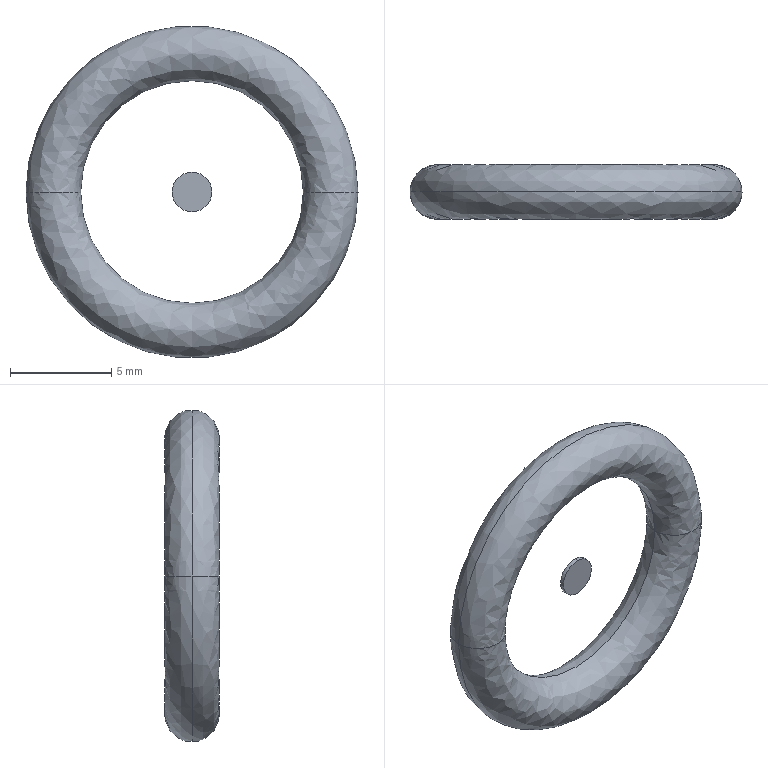Part | STEP file | 20501 | 2 solids | 8 faces | box 16.4 x 2.7 x 16.4 mm | volume 247.033 mm3 | spline 4 | cylinder 2 | plane 2 | commonest cylinder face diameters 1.965 x2
STEP:
#1=CARTESIAN_POINT('',(0.,0.,0.));
#2=DIRECTION('',(0.,0.,1.));
#3=DIRECTION('',(1.,0.,0.));
#4=AXIS2_PLACEMENT_3D('',#1,#2,#3);
#5=CARTESIAN_POINT('',(-5.5,0.,0.));
#6=VERTEX_POINT('',#5);
#7=CARTESIAN_POINT('',(5.5,0.,0.));
#8=VERTEX_POINT('',#7);
#9=CARTESIAN_POINT('',(0.,0.,0.));
#10=DIRECTION('',(0.,1.,0.));
#11=DIRECTION('',(1.,0.,0.));
#12=AXIS2_PLACEMENT_3D('',#9,#10,#11);
#13=CIRCLE('',#12,5.5);
#14=CARTESIAN_POINT('',(-5.5,0.,0.));
#15=CARTESIAN_POINT('',(-5.5,0.,11.));
#16=CARTESIAN_POINT('',(5.5,0.,11.));
#17=CARTESIAN_POINT('',(5.5,0.,0.));
#18=CARTESIAN_POINT('',(-5.5,2.7,0.));
#19=CARTESIAN_POINT('',(-5.5,2.7,11.));
#20=CARTESIAN_POINT('',(5.5,2.7,11.));
#21=CARTESIAN_POINT('',(5.5,2.7,0.));
#22=CARTESIAN_POINT('',(-8.2,2.7,0.));
#23=CARTESIAN_POINT('',(-8.2,2.7,16.4));
#24=CARTESIAN_POINT('',(8.2,2.7,16.4));
#25=CARTESIAN_POINT('',(8.2,2.7,0.));
#26=CARTESIAN_POINT('',(-8.2,0.,0.));
#27=CARTESIAN_POINT('',(-8.2,0.,16.4));
#28=CARTESIAN_POINT('',(8.2,0.,16.4));
#29=CARTESIAN_POINT('',(8.2,0.,0.));
#30=(BOUNDED_SURFACE()B_SPLINE_SURFACE(3,3,((#14,#15,#16,#17),(#18,#19,#20,#21),(#22,#23,#24,#25),(#26,#27,#28,#29)),.UNSPECIFIED.,.F.,.F.,.F.)B_SPLINE_SURFACE_WITH_KNOTS((4,4),(4,4),(0.,1.),(0.,1.),.PIECEWISE_BEZIER_KNOTS.)GEOMETRIC_REPRESENTATION_ITEM()RATIONAL_B_SPLINE_SURFACE(((1.,0.3333,0.3333,1.),(0.3333,0.1111,0.1111,0.3333),(0.3333,0.1111,0.1111,0.3333),(1.,0.3333,0.3333,1.)))REPRESENTATION_ITEM('')SURFACE());
#31=CARTESIAN_POINT('',(0.,0.));
#32=CARTESIAN_POINT('',(0.,0.02375));
#33=CARTESIAN_POINT('',(0.,0.06805));
#34=CARTESIAN_POINT('',(0.,0.1267));
#35=CARTESIAN_POINT('',(0.,0.1794));
#36=CARTESIAN_POINT('',(0.,0.2276));
#37=CARTESIAN_POINT('',(0.,0.2721));
#38=CARTESIAN_POINT('',(0.,0.3139));
#39=CARTESIAN_POINT('',(0.,0.3535));
#40=CARTESIAN_POINT('',(0.,0.3914));
#41=CARTESIAN_POINT('',(0.,0.4282));
#42=CARTESIAN_POINT('',(0.,0.4643));
#43=CARTESIAN_POINT('',(0.,0.5));
#44=CARTESIAN_POINT('',(0.,0.5357));
#45=CARTESIAN_POINT('',(0.,0.5718));
#46=CARTESIAN_POINT('',(0.,0.6086));
#47=CARTESIAN_POINT('',(0.,0.6465));
#48=CARTESIAN_POINT('',(0.,0.6861));
#49=CARTESIAN_POINT('',(0.,0.7279));
#50=CARTESIAN_POINT('',(0.,0.7724));
#51=CARTESIAN_POINT('',(0.,0.8206));
#52=CARTESIAN_POINT('',(0.,0.8733));
#53=CARTESIAN_POINT('',(0.,0.9319));
#54=CARTESIAN_POINT('',(0.,0.9763));
#55=CARTESIAN_POINT('',(0.,1.));
#56=B_SPLINE_CURVE_WITH_KNOTS('',3,(#31,#32,#33,#34,#35,#36,#37,#38,#39,#40,#41,#42,#43,#44,#45,#46,#47,#48,#49,#50,#51,#52,#53,#54,#55),.UNSPECIFIED.,.F.,.F.,(4,1,1,1,1,1,1,1,1,1,1,1,1,1,1,1,1,1,1,1,1,1,4),(3.142,3.284,3.427,3.57,3.713,3.856,3.998,4.141,4.284,4.427,4.57,4.712,4.855,4.998,5.141,5.284,5.426,5.569,5.712,5.855,5.998,6.14,6.283),.QUASI_UNIFORM_KNOTS.);
#57=(GEOMETRIC_REPRESENTATION_CONTEXT(2)PARAMETRIC_REPRESENTATION_CONTEXT()REPRESENTATION_CONTEXT('',''));
#58=DEFINITIONAL_REPRESENTATION('',(#56),#57);
#59=PCURVE('',#30,#58);
#60=CARTESIAN_POINT('',(-8.2,0.,0.));
#61=CARTESIAN_POINT('',(-8.2,0.,16.4));
#62=CARTESIAN_POINT('',(8.2,0.,16.4));
#63=CARTESIAN_POINT('',(8.2,0.,0.));
#64=CARTESIAN_POINT('',(-8.2,-2.7,0.));
#65=CARTESIAN_POINT('',(-8.2,-2.7,16.4));
#66=CARTESIAN_POINT('',(8.2,-2.7,16.4));
#67=CARTESIAN_POINT('',(8.2,-2.7,0.));
#68=CARTESIAN_POINT('',(-5.5,-2.7,0.));
#69=CARTESIAN_POINT('',(-5.5,-2.7,11.));
#70=CARTESIAN_POINT('',(5.5,-2.7,11.));
#71=CARTESIAN_POINT('',(5.5,-2.7,0.));
#72=CARTESIAN_POINT('',(-5.5,0.,0.));
#73=CARTESIAN_POINT('',(-5.5,0.,11.));
#74=CARTESIAN_POINT('',(5.5,0.,11.));
#75=CARTESIAN_POINT('',(5.5,0.,0.));
#76=(BOUNDED_SURFACE()B_SPLINE_SURFACE(3,3,((#60,#61,#62,#63),(#64,#65,#66,#67),(#68,#69,#70,#71),(#72,#73,#74,#75)),.UNSPECIFIED.,.F.,.F.,.F.)B_SPLINE_SURFACE_WITH_KNOTS((4,4),(4,4),(0.,1.),(0.,1.),.PIECEWISE_BEZIER_KNOTS.)GEOMETRIC_REPRESENTATION_ITEM()RATIONAL_B_SPLINE_SURFACE(((1.,0.3333,0.3333,1.),(0.3333,0.1111,0.1111,0.3333),(0.3333,0.1111,0.1111,0.3333),(1.,0.3333,0.3333,1.)))REPRESENTATION_ITEM('')SURFACE());
#77=CARTESIAN_POINT('',(1.,0.));
#78=CARTESIAN_POINT('',(1.,0.02375));
#79=CARTESIAN_POINT('',(1.,0.06805));
#80=CARTESIAN_POINT('',(1.,0.1267));
#81=CARTESIAN_POINT('',(1.,0.1794));
#82=CARTESIAN_POINT('',(1.,0.2276));
#83=CARTESIAN_POINT('',(1.,0.2721));
#84=CARTESIAN_POINT('',(1.,0.3139));
#85=CARTESIAN_POINT('',(1.,0.3535));
#86=CARTESIAN_POINT('',(1.,0.3914));
#87=CARTESIAN_POINT('',(1.,0.4282));
#88=CARTESIAN_POINT('',(1.,0.4643));
#89=CARTESIAN_POINT('',(1.,0.5));
#90=CARTESIAN_POINT('',(1.,0.5357));
#91=CARTESIAN_POINT('',(1.,0.5718));
#92=CARTESIAN_POINT('',(1.,0.6086));
#93=CARTESIAN_POINT('',(1.,0.6465));
#94=CARTESIAN_POINT('',(1.,0.6861));
#95=CARTESIAN_POINT('',(1.,0.7279));
#96=CARTESIAN_POINT('',(1.,0.7724));
#97=CARTESIAN_POINT('',(1.,0.8206));
#98=CARTESIAN_POINT('',(1.,0.8733));
#99=CARTESIAN_POINT('',(1.,0.9319));
#100=CARTESIAN_POINT('',(1.,0.9763));
#101=CARTESIAN_POINT('',(1.,1.));
#102=B_SPLINE_CURVE_WITH_KNOTS('',3,(#77,#78,#79,#80,#81,#82,#83,#84,#85,#86,#87,#88,#89,#90,#91,#92,#93,#94,#95,#96,#97,#98,#99,#100,#101),.UNSPECIFIED.,.F.,.F.,(4,1,1,1,1,1,1,1,1,1,1,1,1,1,1,1,1,1,1,1,1,1,4),(3.142,3.284,3.427,3.57,3.713,3.856,3.998,4.141,4.284,4.427,4.57,4.712,4.855,4.998,5.141,5.284,5.426,5.569,5.712,5.855,5.998,6.14,6.283),.QUASI_UNIFORM_KNOTS.);
#103=(GEOMETRIC_REPRESENTATION_CONTEXT(2)PARAMETRIC_REPRESENTATION_CONTEXT()REPRESENTATION_CONTEXT('',''));
#104=DEFINITIONAL_REPRESENTATION('',(#102),#103);
#105=PCURVE('',#76,#104);
#106=SURFACE_CURVE('',#13,(#59,#105),.PCURVE_S1.);
#107=EDGE_CURVE('',#6,#8,#106,.T.);
#108=ORIENTED_EDGE('',*,*,#107,.F.);
#109=CARTESIAN_POINT('',(-8.2,0.,0.));
#110=VERTEX_POINT('',#109);
#111=CARTESIAN_POINT('',(-6.85,0.,0.));
#112=DIRECTION('',(0.,0.,1.));
#113=DIRECTION('',(-1.,0.,0.));
#114=AXIS2_PLACEMENT_3D('',#111,#112,#113);
#115=CIRCLE('',#114,1.35);
#116=CARTESIAN_POINT('',(0.,0.));
#117=CARTESIAN_POINT('',(0.02375,0.));
#118=CARTESIAN_POINT('',(0.06805,0.));
#119=CARTESIAN_POINT('',(0.1267,0.));
#120=CARTESIAN_POINT('',(0.1794,0.));
#121=CARTESIAN_POINT('',(0.2276,0.));
#122=CARTESIAN_POINT('',(0.2721,0.));
#123=CARTESIAN_POINT('',(0.3139,0.));
#124=CARTESIAN_POINT('',(0.3535,0.));
#125=CARTESIAN_POINT('',(0.3914,0.));
#126=CARTESIAN_POINT('',(0.4282,0.));
#127=CARTESIAN_POINT('',(0.4643,0.));
#128=CARTESIAN_POINT('',(0.5,0.));
#129=CARTESIAN_POINT('',(0.5357,0.));
#130=CARTESIAN_POINT('',(0.5718,0.));
#131=CARTESIAN_POINT('',(0.6086,0.));
#132=CARTESIAN_POINT('',(0.6465,0.));
#133=CARTESIAN_POINT('',(0.6861,0.));
#134=CARTESIAN_POINT('',(0.7279,0.));
#135=CARTESIAN_POINT('',(0.7724,0.));
#136=CARTESIAN_POINT('',(0.8206,0.));
#137=CARTESIAN_POINT('',(0.8733,0.));
#138=CARTESIAN_POINT('',(0.9319,0.));
#139=CARTESIAN_POINT('',(0.9763,0.));
#140=CARTESIAN_POINT('',(1.,0.));
#141=B_SPLINE_CURVE_WITH_KNOTS('',3,(#116,#117,#118,#119,#120,#121,#122,#123,#124,#125,#126,#127,#128,#129,#130,#131,#132,#133,#134,#135,#136,#137,#138,#139,#140),.UNSPECIFIED.,.F.,.F.,(4,1,1,1,1,1,1,1,1,1,1,1,1,1,1,1,1,1,1,1,1,1,4),(3.142,3.284,3.427,3.57,3.713,3.856,3.998,4.141,4.284,4.427,4.57,4.712,4.855,4.998,5.141,5.284,5.426,5.569,5.712,5.855,5.998,6.14,6.283),.QUASI_UNIFORM_KNOTS.);
#142=(GEOMETRIC_REPRESENTATION_CONTEXT(2)PARAMETRIC_REPRESENTATION_CONTEXT()REPRESENTATION_CONTEXT('',''));
#143=DEFINITIONAL_REPRESENTATION('',(#141),#142);
#144=PCURVE('',#30,#143);
#145=CARTESIAN_POINT('',(5.5,0.,0.));
#146=CARTESIAN_POINT('',(5.5,0.,-11.));
#147=CARTESIAN_POINT('',(-5.5,0.,-11.));
#148=CARTESIAN_POINT('',(-5.5,0.,0.));
#149=CARTESIAN_POINT('',(5.5,2.7,0.));
#150=CARTESIAN_POINT('',(5.5,2.7,-11.));
#151=CARTESIAN_POINT('',(-5.5,2.7,-11.));
#152=CARTESIAN_POINT('',(-5.5,2.7,0.));
#153=CARTESIAN_POINT('',(8.2,2.7,0.));
#154=CARTESIAN_POINT('',(8.2,2.7,-16.4));
#155=CARTESIAN_POINT('',(-8.2,2.7,-16.4));
#156=CARTESIAN_POINT('',(-8.2,2.7,0.));
#157=CARTESIAN_POINT('',(8.2,0.,0.));
#158=CARTESIAN_POINT('',(8.2,0.,-16.4));
#159=CARTESIAN_POINT('',(-8.2,0.,-16.4));
#160=CARTESIAN_POINT('',(-8.2,0.,0.));
#161=(BOUNDED_SURFACE()B_SPLINE_SURFACE(3,3,((#145,#146,#147,#148),(#149,#150,#151,#152),(#153,#154,#155,#156),(#157,#158,#159,#160)),.UNSPECIFIED.,.F.,.F.,.F.)B_SPLINE_SURFACE_WITH_KNOTS((4,4),(4,4),(0.,1.),(0.,1.),.PIECEWISE_BEZIER_KNOTS.)GEOMETRIC_REPRESENTATION_ITEM()RATIONAL_B_SPLINE_SURFACE(((1.,0.3333,0.3333,1.),(0.3333,0.1111,0.1111,0.3333),(0.3333,0.1111,0.1111,0.3333),(1.,0.3333,0.3333,1.)))REPRESENTATION_ITEM('')SURFACE());
#162=CARTESIAN_POINT('',(0.,1.));
#163=CARTESIAN_POINT('',(0.02375,1.));
#164=CARTESIAN_POINT('',(0.06805,1.));
#165=CARTESIAN_POINT('',(0.1267,1.));
#166=CARTESIAN_POINT('',(0.1794,1.));
#167=CARTESIAN_POINT('',(0.2276,1.));
#168=CARTESIAN_POINT('',(0.2721,1.));
#169=CARTESIAN_POINT('',(0.3139,1.));
#170=CARTESIAN_POINT('',(0.3535,1.));
#171=CARTESIAN_POINT('',(0.3914,1.));
#172=CARTESIAN_POINT('',(0.4282,1.));
#173=CARTESIAN_POINT('',(0.4643,1.));
#174=CARTESIAN_POINT('',(0.5,1.));
#175=CARTESIAN_POINT('',(0.5357,1.));
#176=CARTESIAN_POINT('',(0.5718,1.));
#177=CARTESIAN_POINT('',(0.6086,1.));
#178=CARTESIAN_POINT('',(0.6465,1.));
#179=CARTESIAN_POINT('',(0.6861,1.));
#180=CARTESIAN_POINT('',(0.7279,1.));
#181=CARTESIAN_POINT('',(0.7724,1.));
#182=CARTESIAN_POINT('',(0.8206,1.));
#183=CARTESIAN_POINT('',(0.8733,1.));
#184=CARTESIAN_POINT('',(0.9319,1.));
#185=CARTESIAN_POINT('',(0.9763,1.));
#186=CARTESIAN_POINT('',(1.,1.));
#187=B_SPLINE_CURVE_WITH_KNOTS('',3,(#162,#163,#164,#165,#166,#167,#168,#169,#170,#171,#172,#173,#174,#175,#176,#177,#178,#179,#180,#181,#182,#183,#184,#185,#186),.UNSPECIFIED.,.F.,.F.,(4,1,1,1,1,1,1,1,1,1,1,1,1,1,1,1,1,1,1,1,1,1,4),(3.142,3.284,3.427,3.57,3.713,3.856,3.998,4.141,4.284,4.427,4.57,4.712,4.855,4.998,5.141,5.284,5.426,5.569,5.712,5.855,5.998,6.14,6.283),.QUASI_UNIFORM_KNOTS.);
#188=(GEOMETRIC_REPRESENTATION_CONTEXT(2)PARAMETRIC_REPRESENTATION_CONTEXT()REPRESENTATION_CONTEXT('',''));
#189=DEFINITIONAL_REPRESENTATION('',(#187),#188);
#190=PCURVE('',#161,#189);
#191=SURFACE_CURVE('',#115,(#144,#190),.PCURVE_S1.);
#192=EDGE_CURVE('',#6,#110,#191,.T.);
#193=ORIENTED_EDGE('',*,*,#192,.T.);
#194=CARTESIAN_POINT('',(8.2,0.,0.));
#195=VERTEX_POINT('',#194);
#196=CARTESIAN_POINT('',(0.,0.,0.));
#197=DIRECTION('',(0.,1.,0.));
#198=DIRECTION('',(1.,0.,0.));
#199=AXIS2_PLACEMENT_3D('',#196,#197,#198);
#200=CIRCLE('',#199,8.2);
#201=CARTESIAN_POINT('',(1.,0.));
#202=CARTESIAN_POINT('',(1.,0.02375));
#203=CARTESIAN_POINT('',(1.,0.06805));
#204=CARTESIAN_POINT('',(1.,0.1267));
#205=CARTESIAN_POINT('',(1.,0.1794));
#206=CARTESIAN_POINT('',(1.,0.2276));
#207=CARTESIAN_POINT('',(1.,0.2721));
#208=CARTESIAN_POINT('',(1.,0.3139));
#209=CARTESIAN_POINT('',(1.,0.3535));
#210=CARTESIAN_POINT('',(1.,0.3914));
#211=CARTESIAN_POINT('',(1.,0.4282));
#212=CARTESIAN_POINT('',(1.,0.4643));
#213=CARTESIAN_POINT('',(1.,0.5));
#214=CARTESIAN_POINT('',(1.,0.5357));
#215=CARTESIAN_POINT('',(1.,0.5718));
#216=CARTESIAN_POINT('',(1.,0.6086));
#217=CARTESIAN_POINT('',(1.,0.6465));
#218=CARTESIAN_POINT('',(1.,0.6861));
#219=CARTESIAN_POINT('',(1.,0.7279));
#220=CARTESIAN_POINT('',(1.,0.7724));
#221=CARTESIAN_POINT('',(1.,0.8206));
#222=CARTESIAN_POINT('',(1.,0.8733));
#223=CARTESIAN_POINT('',(1.,0.9319));
#224=CARTESIAN_POINT('',(1.,0.9763));
#225=CARTESIAN_POINT('',(1.,1.));
#226=B_SPLINE_CURVE_WITH_KNOTS('',3,(#201,#202,#203,#204,#205,#206,#207,#208,#209,#210,#211,#212,#213,#214,#215,#216,#217,#218,#219,#220,#221,#222,#223,#224,#225),.UNSPECIFIED.,.F.,.F.,(4,1,1,1,1,1,1,1,1,1,1,1,1,1,1,1,1,1,1,1,1,1,4),(3.142,3.284,3.427,3.57,3.713,3.856,3.998,4.141,4.284,4.427,4.57,4.712,4.855,4.998,5.141,5.284,5.426,5.569,5.712,5.855,5.998,6.14,6.283),.QUASI_UNIFORM_KNOTS.);
#227=(GEOMETRIC_REPRESENTATION_CONTEXT(2)PARAMETRIC_REPRESENTATION_CONTEXT()REPRESENTATION_CONTEXT('',''));
#228=DEFINITIONAL_REPRESENTATION('',(#226),#227);
#229=PCURVE('',#30,#228);
#230=CARTESIAN_POINT('',(0.,0.));
#231=CARTESIAN_POINT('',(0.,0.02375));
#232=CARTESIAN_POINT('',(0.,0.06805));
#233=CARTESIAN_POINT('',(0.,0.1267));
#234=CARTESIAN_POINT('',(0.,0.1794));
#235=CARTESIAN_POINT('',(0.,0.2276));
#236=CARTESIAN_POINT('',(0.,0.2721));
#237=CARTESIAN_POINT('',(0.,0.3139));
#238=CARTESIAN_POINT('',(0.,0.3535));
#239=CARTESIAN_POINT('',(0.,0.3914));
#240=CARTESIAN_POINT('',(0.,0.4282));
#241=CARTESIAN_POINT('',(0.,0.4643));
#242=CARTESIAN_POINT('',(0.,0.5));
#243=CARTESIAN_POINT('',(0.,0.5357));
#244=CARTESIAN_POINT('',(0.,0.5718));
#245=CARTESIAN_POINT('',(0.,0.6086));
#246=CARTESIAN_POINT('',(0.,0.6465));
#247=CARTESIAN_POINT('',(0.,0.6861));
#248=CARTESIAN_POINT('',(0.,0.7279));
#249=CARTESIAN_POINT('',(0.,0.7724));
#250=CARTESIAN_POINT('',(0.,0.8206));
#251=CARTESIAN_POINT('',(0.,0.8733));
#252=CARTESIAN_POINT('',(0.,0.9319));
#253=CARTESIAN_POINT('',(0.,0.9763));
#254=CARTESIAN_POINT('',(0.,1.));
#255=B_SPLINE_CURVE_WITH_KNOTS('',3,(#230,#231,#232,#233,#234,#235,#236,#237,#238,#239,#240,#241,#242,#243,#244,#245,#246,#247,#248,#249,#250,#251,#252,#253,#254),.UNSPECIFIED.,.F.,.F.,(4,1,1,1,1,1,1,1,1,1,1,1,1,1,1,1,1,1,1,1,1,1,4),(3.142,3.284,3.427,3.57,3.713,3.856,3.998,4.141,4.284,4.427,4.57,4.712,4.855,4.998,5.141,5.284,5.426,5.569,5.712,5.855,5.998,6.14,6.283),.QUASI_UNIFORM_KNOTS.);
#256=(GEOMETRIC_REPRESENTATION_CONTEXT(2)PARAMETRIC_REPRESENTATION_CONTEXT()REPRESENTATION_CONTEXT('',''));
#257=DEFINITIONAL_REPRESENTATION('',(#255),#256);
#258=PCURVE('',#76,#257);
#259=SURFACE_CURVE('',#200,(#229,#258),.PCURVE_S1.);
#260=EDGE_CURVE('',#110,#195,#259,.T.);
#261=ORIENTED_EDGE('',*,*,#260,.T.);
#262=CARTESIAN_POINT('',(6.85,0.,0.));
#263=DIRECTION('',(0.,0.,-1.));
#264=DIRECTION('',(1.,0.,0.));
#265=AXIS2_PLACEMENT_3D('',#262,#263,#264);
#266=CIRCLE('',#265,1.35);
#267=CARTESIAN_POINT('',(0.,1.));
#268=CARTESIAN_POINT('',(0.02375,1.));
#269=CARTESIAN_POINT('',(0.06805,1.));
#270=CARTESIAN_POINT('',(0.1267,1.));
#271=CARTESIAN_POINT('',(0.1794,1.));
#272=CARTESIAN_POINT('',(0.2276,1.));
#273=CARTESIAN_POINT('',(0.2721,1.));
#274=CARTESIAN_POINT('',(0.3139,1.));
#275=CARTESIAN_POINT('',(0.3535,1.));
#276=CARTESIAN_POINT('',(0.3914,1.));
#277=CARTESIAN_POINT('',(0.4282,1.));
#278=CARTESIAN_POINT('',(0.4643,1.));
#279=CARTESIAN_POINT('',(0.5,1.));
#280=CARTESIAN_POINT('',(0.5357,1.));
#281=CARTESIAN_POINT('',(0.5718,1.));
#282=CARTESIAN_POINT('',(0.6086,1.));
#283=CARTESIAN_POINT('',(0.6465,1.));
#284=CARTESIAN_POINT('',(0.6861,1.));
#285=CARTESIAN_POINT('',(0.7279,1.));
#286=CARTESIAN_POINT('',(0.7724,1.));
#287=CARTESIAN_POINT('',(0.8206,1.));
#288=CARTESIAN_POINT('',(0.8733,1.));
#289=CARTESIAN_POINT('',(0.9319,1.));
#290=CARTESIAN_POINT('',(0.9763,1.));
#291=CARTESIAN_POINT('',(1.,1.));
#292=B_SPLINE_CURVE_WITH_KNOTS('',3,(#267,#268,#269,#270,#271,#272,#273,#274,#275,#276,#277,#278,#279,#280,#281,#282,#283,#284,#285,#286,#287,#288,#289,#290,#291),.UNSPECIFIED.,.F.,.F.,(4,1,1,1,1,1,1,1,1,1,1,1,1,1,1,1,1,1,1,1,1,1,4),(3.142,3.284,3.427,3.57,3.713,3.856,3.998,4.141,4.284,4.427,4.57,4.712,4.855,4.998,5.141,5.284,5.426,5.569,5.712,5.855,5.998,6.14,6.283),.QUASI_UNIFORM_KNOTS.);
#293=(GEOMETRIC_REPRESENTATION_CONTEXT(2)PARAMETRIC_REPRESENTATION_CONTEXT()REPRESENTATION_CONTEXT('',''));
#294=DEFINITIONAL_REPRESENTATION('',(#292),#293);
#295=PCURVE('',#30,#294);
#296=CARTESIAN_POINT('',(0.,0.));
#297=CARTESIAN_POINT('',(0.02375,0.));
#298=CARTESIAN_POINT('',(0.06805,0.));
#299=CARTESIAN_POINT('',(0.1267,0.));
#300=CARTESIAN_POINT('',(0.1794,0.));
#301=CARTESIAN_POINT('',(0.2276,0.));
#302=CARTESIAN_POINT('',(0.2721,0.));
#303=CARTESIAN_POINT('',(0.3139,0.));
#304=CARTESIAN_POINT('',(0.3535,0.));
#305=CARTESIAN_POINT('',(0.3914,0.));
#306=CARTESIAN_POINT('',(0.4282,0.));
#307=CARTESIAN_POINT('',(0.4643,0.));
#308=CARTESIAN_POINT('',(0.5,0.));
#309=CARTESIAN_POINT('',(0.5357,0.));
#310=CARTESIAN_POINT('',(0.5718,0.));
#311=CARTESIAN_POINT('',(0.6086,0.));
#312=CARTESIAN_POINT('',(0.6465,0.));
#313=CARTESIAN_POINT('',(0.6861,0.));
#314=CARTESIAN_POINT('',(0.7279,0.));
#315=CARTESIAN_POINT('',(0.7724,0.));
#316=CARTESIAN_POINT('',(0.8206,0.));
#317=CARTESIAN_POINT('',(0.8733,0.));
#318=CARTESIAN_POINT('',(0.9319,0.));
#319=CARTESIAN_POINT('',(0.9763,0.));
#320=CARTESIAN_POINT('',(1.,0.));
#321=B_SPLINE_CURVE_WITH_KNOTS('',3,(#296,#297,#298,#299,#300,#301,#302,#303,#304,#305,#306,#307,#308,#309,#310,#311,#312,#313,#314,#315,#316,#317,#318,#319,#320),.UNSPECIFIED.,.F.,.F.,(4,1,1,1,1,1,1,1,1,1,1,1,1,1,1,1,1,1,1,1,1,1,4),(3.142,3.284,3.427,3.57,3.713,3.856,3.998,4.141,4.284,4.427,4.57,4.712,4.855,4.998,5.141,5.284,5.426,5.569,5.712,5.855,5.998,6.14,6.283),.QUASI_UNIFORM_KNOTS.);
#322=(GEOMETRIC_REPRESENTATION_CONTEXT(2)PARAMETRIC_REPRESENTATION_CONTEXT()REPRESENTATION_CONTEXT('',''));
#323=DEFINITIONAL_REPRESENTATION('',(#321),#322);
#324=PCURVE('',#161,#323);
#325=SURFACE_CURVE('',#266,(#295,#324),.PCURVE_S1.);
#326=EDGE_CURVE('',#8,#195,#325,.T.);
#327=ORIENTED_EDGE('',*,*,#326,.F.);
#328=EDGE_LOOP('',(#108,#193,#261,#327));
#329=FACE_BOUND('',#328,.T.);
#330=ADVANCED_FACE('',(#329),#30,.T.);
#331=ORIENTED_EDGE('',*,*,#260,.F.);
#332=CARTESIAN_POINT('',(-6.85,0.,0.));
#333=DIRECTION('',(0.,0.,1.));
#334=DIRECTION('',(-1.,0.,0.));
#335=AXIS2_PLACEMENT_3D('',#332,#333,#334);
#336=CIRCLE('',#335,1.35);
#337=CARTESIAN_POINT('',(0.,0.));
#338=CARTESIAN_POINT('',(0.02375,0.));
#339=CARTESIAN_POINT('',(0.06805,0.));
#340=CARTESIAN_POINT('',(0.1267,0.));
#341=CARTESIAN_POINT('',(0.1794,0.));
#342=CARTESIAN_POINT('',(0.2276,0.));
#343=CARTESIAN_POINT('',(0.2721,0.));
#344=CARTESIAN_POINT('',(0.3139,0.));
#345=CARTESIAN_POINT('',(0.3535,0.));
#346=CARTESIAN_POINT('',(0.3914,0.));
#347=CARTESIAN_POINT('',(0.4282,0.));
#348=CARTESIAN_POINT('',(0.4643,0.));
#349=CARTESIAN_POINT('',(0.5,0.));
#350=CARTESIAN_POINT('',(0.5357,0.));
#351=CARTESIAN_POINT('',(0.5718,0.));
#352=CARTESIAN_POINT('',(0.6086,0.));
#353=CARTESIAN_POINT('',(0.6465,0.));
#354=CARTESIAN_POINT('',(0.6861,0.));
#355=CARTESIAN_POINT('',(0.7279,0.));
#356=CARTESIAN_POINT('',(0.7724,0.));
#357=CARTESIAN_POINT('',(0.8206,0.));
#358=CARTESIAN_POINT('',(0.8733,0.));
#359=CARTESIAN_POINT('',(0.9319,0.));
#360=CARTESIAN_POINT('',(0.9763,0.));
#361=CARTESIAN_POINT('',(1.,0.));
#362=B_SPLINE_CURVE_WITH_KNOTS('',3,(#337,#338,#339,#340,#341,#342,#343,#344,#345,#346,#347,#348,#349,#350,#351,#352,#353,#354,#355,#356,#357,#358,#359,#360,#361),.UNSPECIFIED.,.F.,.F.,(4,1,1,1,1,1,1,1,1,1,1,1,1,1,1,1,1,1,1,1,1,1,4),(0.,0.1428,0.2856,0.4284,0.5712,0.714,0.8568,0.9996,1.142,1.285,1.428,1.571,1.714,1.856,1.999,2.142,2.285,2.428,2.57,2.713,2.856,2.999,3.142),.QUASI_UNIFORM_KNOTS.);
#363=(GEOMETRIC_REPRESENTATION_CONTEXT(2)PARAMETRIC_REPRESENTATION_CONTEXT()REPRESENTATION_CONTEXT('',''));
#364=DEFINITIONAL_REPRESENTATION('',(#362),#363);
#365=PCURVE('',#76,#364);
#366=CARTESIAN_POINT('',(8.2,0.,0.));
#367=CARTESIAN_POINT('',(8.2,0.,-16.4));
#368=CARTESIAN_POINT('',(-8.2,0.,-16.4));
#369=CARTESIAN_POINT('',(-8.2,0.,0.));
#370=CARTESIAN_POINT('',(8.2,-2.7,0.));
#371=CARTESIAN_POINT('',(8.2,-2.7,-16.4));
#372=CARTESIAN_POINT('',(-8.2,-2.7,-16.4));
#373=CARTESIAN_POINT('',(-8.2,-2.7,0.));
#374=CARTESIAN_POINT('',(5.5,-2.7,0.));
#375=CARTESIAN_POINT('',(5.5,-2.7,-11.));
#376=CARTESIAN_POINT('',(-5.5,-2.7,-11.));
#377=CARTESIAN_POINT('',(-5.5,-2.7,0.));
#378=CARTESIAN_POINT('',(5.5,0.,0.));
#379=CARTESIAN_POINT('',(5.5,0.,-11.));
#380=CARTESIAN_POINT('',(-5.5,0.,-11.));
#381=CARTESIAN_POINT('',(-5.5,0.,0.));
#382=(BOUNDED_SURFACE()B_SPLINE_SURFACE(3,3,((#366,#367,#368,#369),(#370,#371,#372,#373),(#374,#375,#376,#377),(#378,#379,#380,#381)),.UNSPECIFIED.,.F.,.F.,.F.)B_SPLINE_SURFACE_WITH_KNOTS((4,4),(4,4),(0.,1.),(0.,1.),.PIECEWISE_BEZIER_KNOTS.)GEOMETRIC_REPRESENTATION_ITEM()RATIONAL_B_SPLINE_SURFACE(((1.,0.3333,0.3333,1.),(0.3333,0.1111,0.1111,0.3333),(0.3333,0.1111,0.1111,0.3333),(1.,0.3333,0.3333,1.)))REPRESENTATION_ITEM('')SURFACE());
#383=CARTESIAN_POINT('',(0.,1.));
#384=CARTESIAN_POINT('',(0.02375,1.));
#385=CARTESIAN_POINT('',(0.06805,1.));
#386=CARTESIAN_POINT('',(0.1267,1.));
#387=CARTESIAN_POINT('',(0.1794,1.));
#388=CARTESIAN_POINT('',(0.2276,1.));
#389=CARTESIAN_POINT('',(0.2721,1.));
#390=CARTESIAN_POINT('',(0.3139,1.));
#391=CARTESIAN_POINT('',(0.3535,1.));
#392=CARTESIAN_POINT('',(0.3914,1.));
#393=CARTESIAN_POINT('',(0.4282,1.));
#394=CARTESIAN_POINT('',(0.4643,1.));
#395=CARTESIAN_POINT('',(0.5,1.));
#396=CARTESIAN_POINT('',(0.5357,1.));
#397=CARTESIAN_POINT('',(0.5718,1.));
#398=CARTESIAN_POINT('',(0.6086,1.));
#399=CARTESIAN_POINT('',(0.6465,1.));
#400=CARTESIAN_POINT('',(0.6861,1.));
#401=CARTESIAN_POINT('',(0.7279,1.));
#402=CARTESIAN_POINT('',(0.7724,1.));
#403=CARTESIAN_POINT('',(0.8206,1.));
#404=CARTESIAN_POINT('',(0.8733,1.));
#405=CARTESIAN_POINT('',(0.9319,1.));
#406=CARTESIAN_POINT('',(0.9763,1.));
#407=CARTESIAN_POINT('',(1.,1.));
#408=B_SPLINE_CURVE_WITH_KNOTS('',3,(#383,#384,#385,#386,#387,#388,#389,#390,#391,#392,#393,#394,#395,#396,#397,#398,#399,#400,#401,#402,#403,#404,#405,#406,#407),.UNSPECIFIED.,.F.,.F.,(4,1,1,1,1,1,1,1,1,1,1,1,1,1,1,1,1,1,1,1,1,1,4),(0.,0.1428,0.2856,0.4284,0.5712,0.714,0.8568,0.9996,1.142,1.285,1.428,1.571,1.714,1.856,1.999,2.142,2.285,2.428,2.57,2.713,2.856,2.999,3.142),.QUASI_UNIFORM_KNOTS.);
#409=(GEOMETRIC_REPRESENTATION_CONTEXT(2)PARAMETRIC_REPRESENTATION_CONTEXT()REPRESENTATION_CONTEXT('',''));
#410=DEFINITIONAL_REPRESENTATION('',(#408),#409);
#411=PCURVE('',#382,#410);
#412=SURFACE_CURVE('',#336,(#365,#411),.PCURVE_S1.);
#413=EDGE_CURVE('',#110,#6,#412,.T.);
#414=ORIENTED_EDGE('',*,*,#413,.T.);
#415=ORIENTED_EDGE('',*,*,#107,.T.);
#416=CARTESIAN_POINT('',(6.85,0.,0.));
#417=DIRECTION('',(0.,0.,-1.));
#418=DIRECTION('',(1.,0.,0.));
#419=AXIS2_PLACEMENT_3D('',#416,#417,#418);
#420=CIRCLE('',#419,1.35);
#421=CARTESIAN_POINT('',(0.,1.));
#422=CARTESIAN_POINT('',(0.02375,1.));
#423=CARTESIAN_POINT('',(0.06805,1.));
#424=CARTESIAN_POINT('',(0.1267,1.));
#425=CARTESIAN_POINT('',(0.1794,1.));
#426=CARTESIAN_POINT('',(0.2276,1.));
#427=CARTESIAN_POINT('',(0.2721,1.));
#428=CARTESIAN_POINT('',(0.3139,1.));
#429=CARTESIAN_POINT('',(0.3535,1.));
#430=CARTESIAN_POINT('',(0.3914,1.));
#431=CARTESIAN_POINT('',(0.4282,1.));
#432=CARTESIAN_POINT('',(0.4643,1.));
#433=CARTESIAN_POINT('',(0.5,1.));
#434=CARTESIAN_POINT('',(0.5357,1.));
#435=CARTESIAN_POINT('',(0.5718,1.));
#436=CARTESIAN_POINT('',(0.6086,1.));
#437=CARTESIAN_POINT('',(0.6465,1.));
#438=CARTESIAN_POINT('',(0.6861,1.));
#439=CARTESIAN_POINT('',(0.7279,1.));
#440=CARTESIAN_POINT('',(0.7724,1.));
#441=CARTESIAN_POINT('',(0.8206,1.));
#442=CARTESIAN_POINT('',(0.8733,1.));
#443=CARTESIAN_POINT('',(0.9319,1.));
#444=CARTESIAN_POINT('',(0.9763,1.));
#445=CARTESIAN_POINT('',(1.,1.));
#446=B_SPLINE_CURVE_WITH_KNOTS('',3,(#421,#422,#423,#424,#425,#426,#427,#428,#429,#430,#431,#432,#433,#434,#435,#436,#437,#438,#439,#440,#441,#442,#443,#444,#445),.UNSPECIFIED.,.F.,.F.,(4,1,1,1,1,1,1,1,1,1,1,1,1,1,1,1,1,1,1,1,1,1,4),(0.,0.1428,0.2856,0.4284,0.5712,0.714,0.8568,0.9996,1.142,1.285,1.428,1.571,1.714,1.856,1.999,2.142,2.285,2.428,2.57,2.713,2.856,2.999,3.142),.QUASI_UNIFORM_KNOTS.);
#447=(GEOMETRIC_REPRESENTATION_CONTEXT(2)PARAMETRIC_REPRESENTATION_CONTEXT()REPRESENTATION_CONTEXT('',''));
#448=DEFINITIONAL_REPRESENTATION('',(#446),#447);
#449=PCURVE('',#76,#448);
#450=CARTESIAN_POINT('',(0.,0.));
#451=CARTESIAN_POINT('',(0.02375,0.));
#452=CARTESIAN_POINT('',(0.06805,0.));
#453=CARTESIAN_POINT('',(0.1267,0.));
#454=CARTESIAN_POINT('',(0.1794,0.));
#455=CARTESIAN_POINT('',(0.2276,0.));
#456=CARTESIAN_POINT('',(0.2721,0.));
#457=CARTESIAN_POINT('',(0.3139,0.));
#458=CARTESIAN_POINT('',(0.3535,0.));
#459=CARTESIAN_POINT('',(0.3914,0.));
#460=CARTESIAN_POINT('',(0.4282,0.));
#461=CARTESIAN_POINT('',(0.4643,0.));
#462=CARTESIAN_POINT('',(0.5,0.));
#463=CARTESIAN_POINT('',(0.5357,0.));
#464=CARTESIAN_POINT('',(0.5718,0.));
#465=CARTESIAN_POINT('',(0.6086,0.));
#466=CARTESIAN_POINT('',(0.6465,0.));
#467=CARTESIAN_POINT('',(0.6861,0.));
#468=CARTESIAN_POINT('',(0.7279,0.));
#469=CARTESIAN_POINT('',(0.7724,0.));
#470=CARTESIAN_POINT('',(0.8206,0.));
#471=CARTESIAN_POINT('',(0.8733,0.));
#472=CARTESIAN_POINT('',(0.9319,0.));
#473=CARTESIAN_POINT('',(0.9763,0.));
#474=CARTESIAN_POINT('',(1.,0.));
#475=B_SPLINE_CURVE_WITH_KNOTS('',3,(#450,#451,#452,#453,#454,#455,#456,#457,#458,#459,#460,#461,#462,#463,#464,#465,#466,#467,#468,#469,#470,#471,#472,#473,#474),.UNSPECIFIED.,.F.,.F.,(4,1,1,1,1,1,1,1,1,1,1,1,1,1,1,1,1,1,1,1,1,1,4),(0.,0.1428,0.2856,0.4284,0.5712,0.714,0.8568,0.9996,1.142,1.285,1.428,1.571,1.714,1.856,1.999,2.142,2.285,2.428,2.57,2.713,2.856,2.999,3.142),.QUASI_UNIFORM_KNOTS.);
#476=(GEOMETRIC_REPRESENTATION_CONTEXT(2)PARAMETRIC_REPRESENTATION_CONTEXT()REPRESENTATION_CONTEXT('',''));
#477=DEFINITIONAL_REPRESENTATION('',(#475),#476);
#478=PCURVE('',#382,#477);
#479=SURFACE_CURVE('',#420,(#449,#478),.PCURVE_S1.);
#480=EDGE_CURVE('',#195,#8,#479,.T.);
#481=ORIENTED_EDGE('',*,*,#480,.F.);
#482=EDGE_LOOP('',(#331,#414,#415,#481));
#483=FACE_BOUND('',#482,.T.);
#484=ADVANCED_FACE('',(#483),#76,.T.);
#485=ORIENTED_EDGE('',*,*,#413,.F.);
#486=CARTESIAN_POINT('',(0.,0.,0.));
#487=DIRECTION('',(0.,1.,0.));
#488=DIRECTION('',(1.,0.,0.));
#489=AXIS2_PLACEMENT_3D('',#486,#487,#488);
#490=CIRCLE('',#489,8.2);
#491=CARTESIAN_POINT('',(0.,0.));
#492=CARTESIAN_POINT('',(0.,0.02375));
#493=CARTESIAN_POINT('',(0.,0.06805));
#494=CARTESIAN_POINT('',(0.,0.1267));
#495=CARTESIAN_POINT('',(0.,0.1794));
#496=CARTESIAN_POINT('',(0.,0.2276));
#497=CARTESIAN_POINT('',(0.,0.2721));
#498=CARTESIAN_POINT('',(0.,0.3139));
#499=CARTESIAN_POINT('',(0.,0.3535));
#500=CARTESIAN_POINT('',(0.,0.3914));
#501=CARTESIAN_POINT('',(0.,0.4282));
#502=CARTESIAN_POINT('',(0.,0.4643));
#503=CARTESIAN_POINT('',(0.,0.5));
#504=CARTESIAN_POINT('',(0.,0.5357));
#505=CARTESIAN_POINT('',(0.,0.5718));
#506=CARTESIAN_POINT('',(0.,0.6086));
#507=CARTESIAN_POINT('',(0.,0.6465));
#508=CARTESIAN_POINT('',(0.,0.6861));
#509=CARTESIAN_POINT('',(0.,0.7279));
#510=CARTESIAN_POINT('',(0.,0.7724));
#511=CARTESIAN_POINT('',(0.,0.8206));
#512=CARTESIAN_POINT('',(0.,0.8733));
#513=CARTESIAN_POINT('',(0.,0.9319));
#514=CARTESIAN_POINT('',(0.,0.9763));
#515=CARTESIAN_POINT('',(0.,1.));
#516=B_SPLINE_CURVE_WITH_KNOTS('',3,(#491,#492,#493,#494,#495,#496,#497,#498,#499,#500,#501,#502,#503,#504,#505,#506,#507,#508,#509,#510,#511,#512,#513,#514,#515),.UNSPECIFIED.,.F.,.F.,(4,1,1,1,1,1,1,1,1,1,1,1,1,1,1,1,1,1,1,1,1,1,4),(0.,0.1428,0.2856,0.4284,0.5712,0.714,0.8568,0.9996,1.142,1.285,1.428,1.571,1.714,1.856,1.999,2.142,2.285,2.428,2.57,2.713,2.856,2.999,3.142),.QUASI_UNIFORM_KNOTS.);
#517=(GEOMETRIC_REPRESENTATION_CONTEXT(2)PARAMETRIC_REPRESENTATION_CONTEXT()REPRESENTATION_CONTEXT('',''));
#518=DEFINITIONAL_REPRESENTATION('',(#516),#517);
#519=PCURVE('',#382,#518);
#520=CARTESIAN_POINT('',(1.,0.));
#521=CARTESIAN_POINT('',(1.,0.02375));
#522=CARTESIAN_POINT('',(1.,0.06805));
#523=CARTESIAN_POINT('',(1.,0.1267));
#524=CARTESIAN_POINT('',(1.,0.1794));
#525=CARTESIAN_POINT('',(1.,0.2276));
#526=CARTESIAN_POINT('',(1.,0.2721));
#527=CARTESIAN_POINT('',(1.,0.3139));
#528=CARTESIAN_POINT('',(1.,0.3535));
#529=CARTESIAN_POINT('',(1.,0.3914));
#530=CARTESIAN_POINT('',(1.,0.4282));
#531=CARTESIAN_POINT('',(1.,0.4643));
#532=CARTESIAN_POINT('',(1.,0.5));
#533=CARTESIAN_POINT('',(1.,0.5357));
#534=CARTESIAN_POINT('',(1.,0.5718));
#535=CARTESIAN_POINT('',(1.,0.6086));
#536=CARTESIAN_POINT('',(1.,0.6465));
#537=CARTESIAN_POINT('',(1.,0.6861));
#538=CARTESIAN_POINT('',(1.,0.7279));
#539=CARTESIAN_POINT('',(1.,0.7724));
#540=CARTESIAN_POINT('',(1.,0.8206));
#541=CARTESIAN_POINT('',(1.,0.8733));
#542=CARTESIAN_POINT('',(1.,0.9319));
#543=CARTESIAN_POINT('',(1.,0.9763));
#544=CARTESIAN_POINT('',(1.,1.));
#545=B_SPLINE_CURVE_WITH_KNOTS('',3,(#520,#521,#522,#523,#524,#525,#526,#527,#528,#529,#530,#531,#532,#533,#534,#535,#536,#537,#538,#539,#540,#541,#542,#543,#544),.UNSPECIFIED.,.F.,.F.,(4,1,1,1,1,1,1,1,1,1,1,1,1,1,1,1,1,1,1,1,1,1,4),(0.,0.1428,0.2856,0.4284,0.5712,0.714,0.8568,0.9996,1.142,1.285,1.428,1.571,1.714,1.856,1.999,2.142,2.285,2.428,2.57,2.713,2.856,2.999,3.142),.QUASI_UNIFORM_KNOTS.);
#546=(GEOMETRIC_REPRESENTATION_CONTEXT(2)PARAMETRIC_REPRESENTATION_CONTEXT()REPRESENTATION_CONTEXT('',''));
#547=DEFINITIONAL_REPRESENTATION('',(#545),#546);
#548=PCURVE('',#161,#547);
#549=SURFACE_CURVE('',#490,(#519,#548),.PCURVE_S1.);
#550=EDGE_CURVE('',#195,#110,#549,.T.);
#551=ORIENTED_EDGE('',*,*,#550,.F.);
#552=ORIENTED_EDGE('',*,*,#480,.T.);
#553=CARTESIAN_POINT('',(0.,0.,0.));
#554=DIRECTION('',(0.,1.,0.));
#555=DIRECTION('',(1.,0.,0.));
#556=AXIS2_PLACEMENT_3D('',#553,#554,#555);
#557=CIRCLE('',#556,5.5);
#558=CARTESIAN_POINT('',(1.,0.));
#559=CARTESIAN_POINT('',(1.,0.02375));
#560=CARTESIAN_POINT('',(1.,0.06805));
#561=CARTESIAN_POINT('',(1.,0.1267));
#562=CARTESIAN_POINT('',(1.,0.1794));
#563=CARTESIAN_POINT('',(1.,0.2276));
#564=CARTESIAN_POINT('',(1.,0.2721));
#565=CARTESIAN_POINT('',(1.,0.3139));
#566=CARTESIAN_POINT('',(1.,0.3535));
#567=CARTESIAN_POINT('',(1.,0.3914));
#568=CARTESIAN_POINT('',(1.,0.4282));
#569=CARTESIAN_POINT('',(1.,0.4643));
#570=CARTESIAN_POINT('',(1.,0.5));
#571=CARTESIAN_POINT('',(1.,0.5357));
#572=CARTESIAN_POINT('',(1.,0.5718));
#573=CARTESIAN_POINT('',(1.,0.6086));
#574=CARTESIAN_POINT('',(1.,0.6465));
#575=CARTESIAN_POINT('',(1.,0.6861));
#576=CARTESIAN_POINT('',(1.,0.7279));
#577=CARTESIAN_POINT('',(1.,0.7724));
#578=CARTESIAN_POINT('',(1.,0.8206));
#579=CARTESIAN_POINT('',(1.,0.8733));
#580=CARTESIAN_POINT('',(1.,0.9319));
#581=CARTESIAN_POINT('',(1.,0.9763));
#582=CARTESIAN_POINT('',(1.,1.));
#583=B_SPLINE_CURVE_WITH_KNOTS('',3,(#558,#559,#560,#561,#562,#563,#564,#565,#566,#567,#568,#569,#570,#571,#572,#573,#574,#575,#576,#577,#578,#579,#580,#581,#582),.UNSPECIFIED.,.F.,.F.,(4,1,1,1,1,1,1,1,1,1,1,1,1,1,1,1,1,1,1,1,1,1,4),(0.,0.1428,0.2856,0.4284,0.5712,0.714,0.8568,0.9996,1.142,1.285,1.428,1.571,1.714,1.856,1.999,2.142,2.285,2.428,2.57,2.713,2.856,2.999,3.142),.QUASI_UNIFORM_KNOTS.);
#584=(GEOMETRIC_REPRESENTATION_CONTEXT(2)PARAMETRIC_REPRESENTATION_CONTEXT()REPRESENTATION_CONTEXT('',''));
#585=DEFINITIONAL_REPRESENTATION('',(#583),#584);
#586=PCURVE('',#382,#585);
#587=CARTESIAN_POINT('',(0.,0.));
#588=CARTESIAN_POINT('',(0.,0.02375));
#589=CARTESIAN_POINT('',(0.,0.06805));
#590=CARTESIAN_POINT('',(0.,0.1267));
#591=CARTESIAN_POINT('',(0.,0.1794));
#592=CARTESIAN_POINT('',(0.,0.2276));
#593=CARTESIAN_POINT('',(0.,0.2721));
#594=CARTESIAN_POINT('',(0.,0.3139));
#595=CARTESIAN_POINT('',(0.,0.3535));
#596=CARTESIAN_POINT('',(0.,0.3914));
#597=CARTESIAN_POINT('',(0.,0.4282));
#598=CARTESIAN_POINT('',(0.,0.4643));
#599=CARTESIAN_POINT('',(0.,0.5));
#600=CARTESIAN_POINT('',(0.,0.5357));
#601=CARTESIAN_POINT('',(0.,0.5718));
#602=CARTESIAN_POINT('',(0.,0.6086));
#603=CARTESIAN_POINT('',(0.,0.6465));
#604=CARTESIAN_POINT('',(0.,0.6861));
#605=CARTESIAN_POINT('',(0.,0.7279));
#606=CARTESIAN_POINT('',(0.,0.7724));
#607=CARTESIAN_POINT('',(0.,0.8206));
#608=CARTESIAN_POINT('',(0.,0.8733));
#609=CARTESIAN_POINT('',(0.,0.9319));
#610=CARTESIAN_POINT('',(0.,0.9763));
#611=CARTESIAN_POINT('',(0.,1.));
#612=B_SPLINE_CURVE_WITH_KNOTS('',3,(#587,#588,#589,#590,#591,#592,#593,#594,#595,#596,#597,#598,#599,#600,#601,#602,#603,#604,#605,#606,#607,#608,#609,#610,#611),.UNSPECIFIED.,.F.,.F.,(4,1,1,1,1,1,1,1,1,1,1,1,1,1,1,1,1,1,1,1,1,1,4),(0.,0.1428,0.2856,0.4284,0.5712,0.714,0.8568,0.9996,1.142,1.285,1.428,1.571,1.714,1.856,1.999,2.142,2.285,2.428,2.57,2.713,2.856,2.999,3.142),.QUASI_UNIFORM_KNOTS.);
#613=(GEOMETRIC_REPRESENTATION_CONTEXT(2)PARAMETRIC_REPRESENTATION_CONTEXT()REPRESENTATION_CONTEXT('',''));
#614=DEFINITIONAL_REPRESENTATION('',(#612),#613);
#615=PCURVE('',#161,#614);
#616=SURFACE_CURVE('',#557,(#586,#615),.PCURVE_S1.);
#617=EDGE_CURVE('',#8,#6,#616,.T.);
#618=ORIENTED_EDGE('',*,*,#617,.T.);
#619=EDGE_LOOP('',(#485,#551,#552,#618));
#620=FACE_BOUND('',#619,.T.);
#621=ADVANCED_FACE('',(#620),#382,.T.);
#622=ORIENTED_EDGE('',*,*,#192,.F.);
#623=ORIENTED_EDGE('',*,*,#617,.F.);
#624=ORIENTED_EDGE('',*,*,#326,.T.);
#625=ORIENTED_EDGE('',*,*,#550,.T.);
#626=EDGE_LOOP('',(#622,#623,#624,#625));
#627=FACE_BOUND('',#626,.T.);
#628=ADVANCED_FACE('',(#627),#161,.T.);
#629=CLOSED_SHELL('',(#330,#484,#621,#628));
#630=MANIFOLD_SOLID_BREP('',#629);
#631=CARTESIAN_POINT('',(0.,0.1,0.9823));
#632=VERTEX_POINT('',#631);
#633=CARTESIAN_POINT('',(0.,0.1,-0.9823));
#634=VERTEX_POINT('',#633);
#635=CARTESIAN_POINT('',(0.,0.1,0.));
#636=DIRECTION('',(0.,1.,0.));
#637=DIRECTION('',(0.,0.,1.));
#638=AXIS2_PLACEMENT_3D('',#635,#636,#637);
#639=CIRCLE('',#638,0.9823);
#640=CARTESIAN_POINT('',(0.,0.1,0.));
#641=DIRECTION('',(0.,-1.,0.));
#642=DIRECTION('',(0.,0.,-1.));
#643=AXIS2_PLACEMENT_3D('',#640,#641,#642);
#644=CYLINDRICAL_SURFACE('',#643,0.9823);
#645=CARTESIAN_POINT('',(3.142,0.));
#646=DIRECTION('',(-1.,0.));
#647=VECTOR('',#646,1.);
#648=LINE('',#645,#647);
#649=(GEOMETRIC_REPRESENTATION_CONTEXT(2)PARAMETRIC_REPRESENTATION_CONTEXT()REPRESENTATION_CONTEXT('',''));
#650=DEFINITIONAL_REPRESENTATION('',(#648),#649);
#651=PCURVE('',#644,#650);
#652=CARTESIAN_POINT('',(0.,0.1,0.));
#653=DIRECTION('',(0.,1.,0.));
#654=DIRECTION('',(0.,0.,1.));
#655=AXIS2_PLACEMENT_3D('',#652,#653,#654);
#656=PLANE('',#655);
#657=CARTESIAN_POINT('',(0.,0.));
#658=DIRECTION('',(1.,0.));
#659=AXIS2_PLACEMENT_2D('',#657,#658);
#660=CIRCLE('',#659,0.9823);
#661=(GEOMETRIC_REPRESENTATION_CONTEXT(2)PARAMETRIC_REPRESENTATION_CONTEXT()REPRESENTATION_CONTEXT('',''));
#662=DEFINITIONAL_REPRESENTATION('',(#660),#661);
#663=PCURVE('',#656,#662);
#664=SURFACE_CURVE('',#639,(#651,#663),.PCURVE_S1.);
#665=EDGE_CURVE('',#632,#634,#664,.T.);
#666=ORIENTED_EDGE('',*,*,#665,.F.);
#667=CARTESIAN_POINT('',(0.,-0.1,0.9823));
#668=VERTEX_POINT('',#667);
#669=CARTESIAN_POINT('',(0.,0.1,0.9823));
#670=DIRECTION('',(0.,-1.,0.));
#671=VECTOR('',#670,1.);
#672=LINE('',#669,#671);
#673=CARTESIAN_POINT('',(3.142,0.));
#674=DIRECTION('',(0.,1.));
#675=VECTOR('',#674,1.);
#676=LINE('',#673,#675);
#677=(GEOMETRIC_REPRESENTATION_CONTEXT(2)PARAMETRIC_REPRESENTATION_CONTEXT()REPRESENTATION_CONTEXT('',''));
#678=DEFINITIONAL_REPRESENTATION('',(#676),#677);
#679=PCURVE('',#644,#678);
#680=CARTESIAN_POINT('',(0.,0.1,0.));
#681=DIRECTION('',(0.,-1.,0.));
#682=DIRECTION('',(0.,0.,-1.));
#683=AXIS2_PLACEMENT_3D('',#680,#681,#682);
#684=CYLINDRICAL_SURFACE('',#683,0.9823);
#685=CARTESIAN_POINT('',(3.142,0.));
#686=DIRECTION('',(0.,1.));
#687=VECTOR('',#686,1.);
#688=LINE('',#685,#687);
#689=(GEOMETRIC_REPRESENTATION_CONTEXT(2)PARAMETRIC_REPRESENTATION_CONTEXT()REPRESENTATION_CONTEXT('',''));
#690=DEFINITIONAL_REPRESENTATION('',(#688),#689);
#691=PCURVE('',#684,#690);
#692=SURFACE_CURVE('',#672,(#679,#691),.PCURVE_S1.);
#693=EDGE_CURVE('',#632,#668,#692,.T.);
#694=ORIENTED_EDGE('',*,*,#693,.T.);
#695=CARTESIAN_POINT('',(0.,-0.1,-0.9823));
#696=VERTEX_POINT('',#695);
#697=CARTESIAN_POINT('',(0.,-0.1,0.));
#698=DIRECTION('',(0.,1.,0.));
#699=DIRECTION('',(0.,0.,1.));
#700=AXIS2_PLACEMENT_3D('',#697,#698,#699);
#701=CIRCLE('',#700,0.9823);
#702=CARTESIAN_POINT('',(3.142,0.2));
#703=DIRECTION('',(-1.,0.));
#704=VECTOR('',#703,1.);
#705=LINE('',#702,#704);
#706=(GEOMETRIC_REPRESENTATION_CONTEXT(2)PARAMETRIC_REPRESENTATION_CONTEXT()REPRESENTATION_CONTEXT('',''));
#707=DEFINITIONAL_REPRESENTATION('',(#705),#706);
#708=PCURVE('',#644,#707);
#709=CARTESIAN_POINT('',(0.,-0.1,0.));
#710=DIRECTION('',(0.,1.,0.));
#711=DIRECTION('',(0.,0.,1.));
#712=AXIS2_PLACEMENT_3D('',#709,#710,#711);
#713=PLANE('',#712);
#714=CARTESIAN_POINT('',(0.,0.));
#715=DIRECTION('',(1.,0.));
#716=AXIS2_PLACEMENT_2D('',#714,#715);
#717=CIRCLE('',#716,0.9823);
#718=(GEOMETRIC_REPRESENTATION_CONTEXT(2)PARAMETRIC_REPRESENTATION_CONTEXT()REPRESENTATION_CONTEXT('',''));
#719=DEFINITIONAL_REPRESENTATION('',(#717),#718);
#720=PCURVE('',#713,#719);
#721=SURFACE_CURVE('',#701,(#708,#720),.PCURVE_S1.);
#722=EDGE_CURVE('',#668,#696,#721,.T.);
#723=ORIENTED_EDGE('',*,*,#722,.T.);
#724=CARTESIAN_POINT('',(0.,0.1,-0.9823));
#725=DIRECTION('',(0.,-1.,0.));
#726=VECTOR('',#725,1.);
#727=LINE('',#724,#726);
#728=CARTESIAN_POINT('',(0.,0.));
#729=DIRECTION('',(0.,1.));
#730=VECTOR('',#729,1.);
#731=LINE('',#728,#730);
#732=(GEOMETRIC_REPRESENTATION_CONTEXT(2)PARAMETRIC_REPRESENTATION_CONTEXT()REPRESENTATION_CONTEXT('',''));
#733=DEFINITIONAL_REPRESENTATION('',(#731),#732);
#734=PCURVE('',#644,#733);
#735=CARTESIAN_POINT('',(6.283,0.));
#736=DIRECTION('',(0.,1.));
#737=VECTOR('',#736,1.);
#738=LINE('',#735,#737);
#739=(GEOMETRIC_REPRESENTATION_CONTEXT(2)PARAMETRIC_REPRESENTATION_CONTEXT()REPRESENTATION_CONTEXT('',''));
#740=DEFINITIONAL_REPRESENTATION('',(#738),#739);
#741=PCURVE('',#684,#740);
#742=SURFACE_CURVE('',#727,(#734,#741),.PCURVE_S1.);
#743=EDGE_CURVE('',#634,#696,#742,.T.);
#744=ORIENTED_EDGE('',*,*,#743,.F.);
#745=EDGE_LOOP('',(#666,#694,#723,#744));
#746=FACE_BOUND('',#745,.T.);
#747=ADVANCED_FACE('',(#746),#644,.T.);
#748=ORIENTED_EDGE('',*,*,#693,.F.);
#749=CARTESIAN_POINT('',(0.,0.1,0.));
#750=DIRECTION('',(0.,1.,0.));
#751=DIRECTION('',(0.,0.,1.));
#752=AXIS2_PLACEMENT_3D('',#749,#750,#751);
#753=CIRCLE('',#752,0.9823);
#754=CARTESIAN_POINT('',(9.425,0.));
#755=DIRECTION('',(-1.,0.));
#756=VECTOR('',#755,1.);
#757=LINE('',#754,#756);
#758=(GEOMETRIC_REPRESENTATION_CONTEXT(2)PARAMETRIC_REPRESENTATION_CONTEXT()REPRESENTATION_CONTEXT('',''));
#759=DEFINITIONAL_REPRESENTATION('',(#757),#758);
#760=PCURVE('',#684,#759);
#761=CARTESIAN_POINT('',(0.,0.));
#762=DIRECTION('',(1.,0.));
#763=AXIS2_PLACEMENT_2D('',#761,#762);
#764=CIRCLE('',#763,0.9823);
#765=(GEOMETRIC_REPRESENTATION_CONTEXT(2)PARAMETRIC_REPRESENTATION_CONTEXT()REPRESENTATION_CONTEXT('',''));
#766=DEFINITIONAL_REPRESENTATION('',(#764),#765);
#767=PCURVE('',#656,#766);
#768=SURFACE_CURVE('',#753,(#760,#767),.PCURVE_S1.);
#769=EDGE_CURVE('',#634,#632,#768,.T.);
#770=ORIENTED_EDGE('',*,*,#769,.F.);
#771=ORIENTED_EDGE('',*,*,#743,.T.);
#772=CARTESIAN_POINT('',(0.,-0.1,0.));
#773=DIRECTION('',(0.,1.,0.));
#774=DIRECTION('',(0.,0.,1.));
#775=AXIS2_PLACEMENT_3D('',#772,#773,#774);
#776=CIRCLE('',#775,0.9823);
#777=CARTESIAN_POINT('',(9.425,0.2));
#778=DIRECTION('',(-1.,0.));
#779=VECTOR('',#778,1.);
#780=LINE('',#777,#779);
#781=(GEOMETRIC_REPRESENTATION_CONTEXT(2)PARAMETRIC_REPRESENTATION_CONTEXT()REPRESENTATION_CONTEXT('',''));
#782=DEFINITIONAL_REPRESENTATION('',(#780),#781);
#783=PCURVE('',#684,#782);
#784=CARTESIAN_POINT('',(0.,0.));
#785=DIRECTION('',(1.,0.));
#786=AXIS2_PLACEMENT_2D('',#784,#785);
#787=CIRCLE('',#786,0.9823);
#788=(GEOMETRIC_REPRESENTATION_CONTEXT(2)PARAMETRIC_REPRESENTATION_CONTEXT()REPRESENTATION_CONTEXT('',''));
#789=DEFINITIONAL_REPRESENTATION('',(#787),#788);
#790=PCURVE('',#713,#789);
#791=SURFACE_CURVE('',#776,(#783,#790),.PCURVE_S1.);
#792=EDGE_CURVE('',#696,#668,#791,.T.);
#793=ORIENTED_EDGE('',*,*,#792,.T.);
#794=EDGE_LOOP('',(#748,#770,#771,#793));
#795=FACE_BOUND('',#794,.T.);
#796=ADVANCED_FACE('',(#795),#684,.T.);
#797=ORIENTED_EDGE('',*,*,#769,.T.);
#798=ORIENTED_EDGE('',*,*,#665,.T.);
#799=EDGE_LOOP('',(#797,#798));
#800=FACE_BOUND('',#799,.T.);
#801=ADVANCED_FACE('',(#800),#656,.T.);
#802=ORIENTED_EDGE('',*,*,#792,.F.);
#803=ORIENTED_EDGE('',*,*,#722,.F.);
#804=EDGE_LOOP('',(#802,#803));
#805=FACE_BOUND('',#804,.T.);
#806=ADVANCED_FACE('',(#805),#713,.F.);
#807=CLOSED_SHELL('',(#747,#796,#801,#806));
#808=MANIFOLD_SOLID_BREP('',#807);
#809=(LENGTH_UNIT()NAMED_UNIT(*)SI_UNIT(.MILLI.,.METRE.));
#810=UNCERTAINTY_MEASURE_WITH_UNIT(LENGTH_MEASURE(0.0000001),#809,'','');
#811=(NAMED_UNIT(*)PLANE_ANGLE_UNIT()SI_UNIT($,.RADIAN.));
#812=(NAMED_UNIT(*)SI_UNIT($,.STERADIAN.)SOLID_ANGLE_UNIT());
#813=(GEOMETRIC_REPRESENTATION_CONTEXT(3)GLOBAL_UNCERTAINTY_ASSIGNED_CONTEXT((#810))GLOBAL_UNIT_ASSIGNED_CONTEXT((#809,#811,#812))REPRESENTATION_CONTEXT('',''));
#814=SHAPE_REPRESENTATION('',(#4,#630,#808),#813);